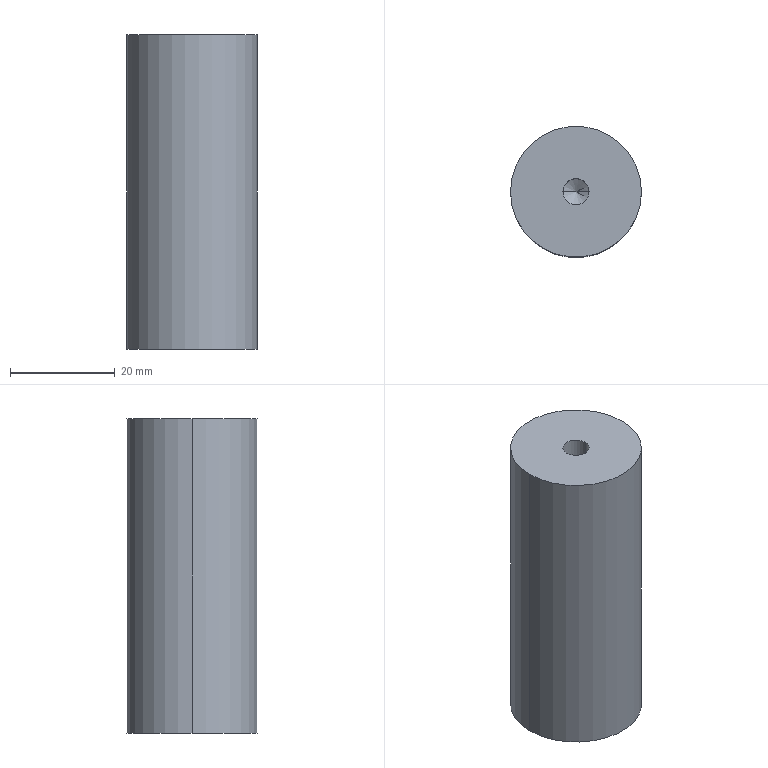Part | SolidWorks | features HoleWzd 2, Extrusion 1 | 1 solid | 12 faces | box 25 x 25 x 60 mm | volume 28844 mm3 | cylinder 6 | cone 4 | plane 2 | commonest cylinder face diameters 5 x4 25 x2
STEP:
#1=CARTESIAN_POINT('',(2.5,0.,15.));
#2=VERTEX_POINT('',#1);
#3=CARTESIAN_POINT('',(-2.5,0.,15.));
#4=VERTEX_POINT('',#3);
#5=CARTESIAN_POINT('',(0.,0.,15.));
#6=DIRECTION('',(0.,0.,-1.));
#7=DIRECTION('',(-1.,0.,0.));
#8=AXIS2_PLACEMENT_3D('',#5,#6,#7);
#9=CIRCLE('',#8,2.5);
#10=EDGE_CURVE('',#2,#4,#9,.T.);
#11=ORIENTED_EDGE('',*,*,#10,.F.);
#12=CARTESIAN_POINT('',(2.5,0.,0.));
#13=VERTEX_POINT('',#12);
#14=CARTESIAN_POINT('',(2.5,0.,0.));
#15=DIRECTION('',(0.,0.,-1.));
#16=VECTOR('',#15,1000.);
#17=LINE('',#14,#16);
#18=EDGE_CURVE('',#2,#13,#17,.T.);
#19=ORIENTED_EDGE('',*,*,#18,.T.);
#20=CARTESIAN_POINT('',(-2.5,0.,0.));
#21=VERTEX_POINT('',#20);
#22=CARTESIAN_POINT('',(0.,0.,0.));
#23=DIRECTION('',(0.,0.,-1.));
#24=DIRECTION('',(-1.,0.,0.));
#25=AXIS2_PLACEMENT_3D('',#22,#23,#24);
#26=CIRCLE('',#25,2.5);
#27=EDGE_CURVE('',#13,#21,#26,.T.);
#28=ORIENTED_EDGE('',*,*,#27,.T.);
#29=CARTESIAN_POINT('',(-2.5,0.,0.));
#30=DIRECTION('',(0.,0.,-1.));
#31=VECTOR('',#30,1000.);
#32=LINE('',#29,#31);
#33=EDGE_CURVE('',#4,#21,#32,.T.);
#34=ORIENTED_EDGE('',*,*,#33,.F.);
#35=EDGE_LOOP('',(#11,#19,#28,#34));
#36=FACE_OUTER_BOUND('',#35,.T.);
#37=CARTESIAN_POINT('',(0.,0.,0.));
#38=DIRECTION('',(0.,0.,-1.));
#39=DIRECTION('',(-1.,0.,0.));
#40=AXIS2_PLACEMENT_3D('',#37,#38,#39);
#41=CYLINDRICAL_SURFACE('',#40,2.5);
#42=ADVANCED_FACE('',(#36),#41,.F.);
#43=CARTESIAN_POINT('',(0.,0.,16.502));
#44=VERTEX_POINT('',#43);
#45=CARTESIAN_POINT('',(-2.5,0.,15.));
#46=DIRECTION('',(-0.8572,0.,-0.515));
#47=VECTOR('',#46,1000.);
#48=LINE('',#45,#47);
#49=EDGE_CURVE('',#44,#4,#48,.T.);
#50=ORIENTED_EDGE('',*,*,#49,.F.);
#51=CARTESIAN_POINT('',(2.5,0.,15.));
#52=DIRECTION('',(0.8572,0.,-0.515));
#53=VECTOR('',#52,1000.);
#54=LINE('',#51,#53);
#55=EDGE_CURVE('',#44,#2,#54,.T.);
#56=ORIENTED_EDGE('',*,*,#55,.T.);
#57=ORIENTED_EDGE('',*,*,#10,.T.);
#58=EDGE_LOOP('',(#50,#56,#57));
#59=FACE_OUTER_BOUND('',#58,.T.);
#60=CARTESIAN_POINT('',(0.,0.,15.));
#61=DIRECTION('',(0.,0.,-1.));
#62=DIRECTION('',(-1.,0.,0.));
#63=AXIS2_PLACEMENT_3D('',#60,#61,#62);
#64=CONICAL_SURFACE('',#63,2.5,1.03);
#65=ADVANCED_FACE('',(#59),#64,.F.);
#66=CARTESIAN_POINT('',(-2.5,0.,45.));
#67=VERTEX_POINT('',#66);
#68=CARTESIAN_POINT('',(2.5,0.,45.));
#69=VERTEX_POINT('',#68);
#70=CARTESIAN_POINT('',(0.,0.,45.));
#71=DIRECTION('',(0.,0.,1.));
#72=DIRECTION('',(1.,0.,0.));
#73=AXIS2_PLACEMENT_3D('',#70,#71,#72);
#74=CIRCLE('',#73,2.5);
#75=EDGE_CURVE('',#67,#69,#74,.T.);
#76=ORIENTED_EDGE('',*,*,#75,.F.);
#77=CARTESIAN_POINT('',(-2.5,0.,60.));
#78=VERTEX_POINT('',#77);
#79=CARTESIAN_POINT('',(-2.5,0.,60.));
#80=DIRECTION('',(0.,0.,1.));
#81=VECTOR('',#80,1000.);
#82=LINE('',#79,#81);
#83=EDGE_CURVE('',#67,#78,#82,.T.);
#84=ORIENTED_EDGE('',*,*,#83,.T.);
#85=CARTESIAN_POINT('',(2.5,0.,60.));
#86=VERTEX_POINT('',#85);
#87=CARTESIAN_POINT('',(0.,0.,60.));
#88=DIRECTION('',(0.,0.,1.));
#89=DIRECTION('',(1.,0.,0.));
#90=AXIS2_PLACEMENT_3D('',#87,#88,#89);
#91=CIRCLE('',#90,2.5);
#92=EDGE_CURVE('',#78,#86,#91,.T.);
#93=ORIENTED_EDGE('',*,*,#92,.T.);
#94=CARTESIAN_POINT('',(2.5,0.,60.));
#95=DIRECTION('',(0.,0.,1.));
#96=VECTOR('',#95,1000.);
#97=LINE('',#94,#96);
#98=EDGE_CURVE('',#69,#86,#97,.T.);
#99=ORIENTED_EDGE('',*,*,#98,.F.);
#100=EDGE_LOOP('',(#76,#84,#93,#99));
#101=FACE_OUTER_BOUND('',#100,.T.);
#102=CARTESIAN_POINT('',(0.,0.,60.));
#103=DIRECTION('',(0.,0.,1.));
#104=DIRECTION('',(1.,0.,0.));
#105=AXIS2_PLACEMENT_3D('',#102,#103,#104);
#106=CYLINDRICAL_SURFACE('',#105,2.5);
#107=ADVANCED_FACE('',(#101),#106,.F.);
#108=CARTESIAN_POINT('',(0.,0.,43.498));
#109=VERTEX_POINT('',#108);
#110=CARTESIAN_POINT('',(2.5,0.,45.));
#111=DIRECTION('',(0.8572,0.,0.515));
#112=VECTOR('',#111,1000.);
#113=LINE('',#110,#112);
#114=EDGE_CURVE('',#109,#69,#113,.T.);
#115=ORIENTED_EDGE('',*,*,#114,.F.);
#116=CARTESIAN_POINT('',(-2.5,0.,45.));
#117=DIRECTION('',(-0.8572,0.,0.515));
#118=VECTOR('',#117,1000.);
#119=LINE('',#116,#118);
#120=EDGE_CURVE('',#109,#67,#119,.T.);
#121=ORIENTED_EDGE('',*,*,#120,.T.);
#122=ORIENTED_EDGE('',*,*,#75,.T.);
#123=EDGE_LOOP('',(#115,#121,#122));
#124=FACE_OUTER_BOUND('',#123,.T.);
#125=CARTESIAN_POINT('',(0.,0.,45.));
#126=DIRECTION('',(0.,0.,1.));
#127=DIRECTION('',(1.,0.,0.));
#128=AXIS2_PLACEMENT_3D('',#125,#126,#127);
#129=CONICAL_SURFACE('',#128,2.5,1.03);
#130=ADVANCED_FACE('',(#124),#129,.F.);
#131=CARTESIAN_POINT('',(12.5,0.,60.));
#132=VERTEX_POINT('',#131);
#133=CARTESIAN_POINT('',(-12.5,0.,60.));
#134=VERTEX_POINT('',#133);
#135=CARTESIAN_POINT('',(0.,0.,60.));
#136=DIRECTION('',(0.,0.,1.));
#137=DIRECTION('',(1.,0.,0.));
#138=AXIS2_PLACEMENT_3D('',#135,#136,#137);
#139=CIRCLE('',#138,12.5);
#140=EDGE_CURVE('',#132,#134,#139,.T.);
#141=ORIENTED_EDGE('',*,*,#140,.F.);
#142=CARTESIAN_POINT('',(12.5,0.,0.));
#143=VERTEX_POINT('',#142);
#144=CARTESIAN_POINT('',(12.5,0.,60.));
#145=DIRECTION('',(0.,0.,-1.));
#146=VECTOR('',#145,1000.);
#147=LINE('',#144,#146);
#148=EDGE_CURVE('',#132,#143,#147,.T.);
#149=ORIENTED_EDGE('',*,*,#148,.T.);
#150=CARTESIAN_POINT('',(-12.5,0.,0.));
#151=VERTEX_POINT('',#150);
#152=CARTESIAN_POINT('',(0.,0.,0.));
#153=DIRECTION('',(0.,0.,1.));
#154=DIRECTION('',(1.,0.,0.));
#155=AXIS2_PLACEMENT_3D('',#152,#153,#154);
#156=CIRCLE('',#155,12.5);
#157=EDGE_CURVE('',#143,#151,#156,.T.);
#158=ORIENTED_EDGE('',*,*,#157,.T.);
#159=CARTESIAN_POINT('',(-12.5,0.,60.));
#160=DIRECTION('',(0.,0.,-1.));
#161=VECTOR('',#160,1000.);
#162=LINE('',#159,#161);
#163=EDGE_CURVE('',#134,#151,#162,.T.);
#164=ORIENTED_EDGE('',*,*,#163,.F.);
#165=EDGE_LOOP('',(#141,#149,#158,#164));
#166=FACE_OUTER_BOUND('',#165,.T.);
#167=CARTESIAN_POINT('',(0.,0.,60.));
#168=DIRECTION('',(0.,0.,-1.));
#169=DIRECTION('',(-1.,0.,0.));
#170=AXIS2_PLACEMENT_3D('',#167,#168,#169);
#171=CYLINDRICAL_SURFACE('',#170,12.5);
#172=ADVANCED_FACE('',(#166),#171,.T.);
#173=ORIENTED_EDGE('',*,*,#148,.F.);
#174=CARTESIAN_POINT('',(0.,0.,60.));
#175=DIRECTION('',(0.,0.,1.));
#176=DIRECTION('',(1.,0.,0.));
#177=AXIS2_PLACEMENT_3D('',#174,#175,#176);
#178=CIRCLE('',#177,12.5);
#179=EDGE_CURVE('',#134,#132,#178,.T.);
#180=ORIENTED_EDGE('',*,*,#179,.F.);
#181=ORIENTED_EDGE('',*,*,#163,.T.);
#182=CARTESIAN_POINT('',(0.,0.,0.));
#183=DIRECTION('',(0.,0.,1.));
#184=DIRECTION('',(1.,0.,0.));
#185=AXIS2_PLACEMENT_3D('',#182,#183,#184);
#186=CIRCLE('',#185,12.5);
#187=EDGE_CURVE('',#151,#143,#186,.T.);
#188=ORIENTED_EDGE('',*,*,#187,.T.);
#189=EDGE_LOOP('',(#173,#180,#181,#188));
#190=FACE_OUTER_BOUND('',#189,.T.);
#191=CARTESIAN_POINT('',(0.,0.,60.));
#192=DIRECTION('',(0.,0.,-1.));
#193=DIRECTION('',(-1.,0.,0.));
#194=AXIS2_PLACEMENT_3D('',#191,#192,#193);
#195=CYLINDRICAL_SURFACE('',#194,12.5);
#196=ADVANCED_FACE('',(#190),#195,.T.);
#197=CARTESIAN_POINT('',(0.,0.,60.));
#198=DIRECTION('',(0.,0.,1.));
#199=DIRECTION('',(1.,0.,0.));
#200=AXIS2_PLACEMENT_3D('',#197,#198,#199);
#201=CIRCLE('',#200,2.5);
#202=EDGE_CURVE('',#86,#78,#201,.T.);
#203=ORIENTED_EDGE('',*,*,#202,.F.);
#204=ORIENTED_EDGE('',*,*,#92,.F.);
#205=EDGE_LOOP('',(#203,#204));
#206=FACE_BOUND('',#205,.T.);
#207=ORIENTED_EDGE('',*,*,#179,.T.);
#208=ORIENTED_EDGE('',*,*,#140,.T.);
#209=EDGE_LOOP('',(#207,#208));
#210=FACE_OUTER_BOUND('',#209,.T.);
#211=CARTESIAN_POINT('',(0.,0.,60.));
#212=DIRECTION('',(0.,0.,1.));
#213=DIRECTION('',(1.,0.,0.));
#214=AXIS2_PLACEMENT_3D('',#211,#212,#213);
#215=PLANE('',#214);
#216=ADVANCED_FACE('',(#206,#210),#215,.T.);
#217=CARTESIAN_POINT('',(0.,0.,0.));
#218=DIRECTION('',(0.,0.,-1.));
#219=DIRECTION('',(-1.,0.,0.));
#220=AXIS2_PLACEMENT_3D('',#217,#218,#219);
#221=CIRCLE('',#220,2.5);
#222=EDGE_CURVE('',#21,#13,#221,.T.);
#223=ORIENTED_EDGE('',*,*,#222,.F.);
#224=ORIENTED_EDGE('',*,*,#27,.F.);
#225=EDGE_LOOP('',(#223,#224));
#226=FACE_BOUND('',#225,.T.);
#227=ORIENTED_EDGE('',*,*,#187,.F.);
#228=ORIENTED_EDGE('',*,*,#157,.F.);
#229=EDGE_LOOP('',(#227,#228));
#230=FACE_OUTER_BOUND('',#229,.T.);
#231=CARTESIAN_POINT('',(0.,0.,0.));
#232=DIRECTION('',(0.,0.,1.));
#233=DIRECTION('',(1.,0.,0.));
#234=AXIS2_PLACEMENT_3D('',#231,#232,#233);
#235=PLANE('',#234);
#236=ADVANCED_FACE('',(#226,#230),#235,.F.);
#237=ORIENTED_EDGE('',*,*,#120,.F.);
#238=ORIENTED_EDGE('',*,*,#114,.T.);
#239=CARTESIAN_POINT('',(0.,0.,45.));
#240=DIRECTION('',(0.,0.,1.));
#241=DIRECTION('',(1.,0.,0.));
#242=AXIS2_PLACEMENT_3D('',#239,#240,#241);
#243=CIRCLE('',#242,2.5);
#244=EDGE_CURVE('',#69,#67,#243,.T.);
#245=ORIENTED_EDGE('',*,*,#244,.T.);
#246=EDGE_LOOP('',(#237,#238,#245));
#247=FACE_OUTER_BOUND('',#246,.T.);
#248=CARTESIAN_POINT('',(0.,0.,45.));
#249=DIRECTION('',(0.,0.,1.));
#250=DIRECTION('',(1.,0.,0.));
#251=AXIS2_PLACEMENT_3D('',#248,#249,#250);
#252=CONICAL_SURFACE('',#251,2.5,1.03);
#253=ADVANCED_FACE('',(#247),#252,.F.);
#254=ORIENTED_EDGE('',*,*,#83,.F.);
#255=ORIENTED_EDGE('',*,*,#244,.F.);
#256=ORIENTED_EDGE('',*,*,#98,.T.);
#257=ORIENTED_EDGE('',*,*,#202,.T.);
#258=EDGE_LOOP('',(#254,#255,#256,#257));
#259=FACE_OUTER_BOUND('',#258,.T.);
#260=CARTESIAN_POINT('',(0.,0.,60.));
#261=DIRECTION('',(0.,0.,1.));
#262=DIRECTION('',(1.,0.,0.));
#263=AXIS2_PLACEMENT_3D('',#260,#261,#262);
#264=CYLINDRICAL_SURFACE('',#263,2.5);
#265=ADVANCED_FACE('',(#259),#264,.F.);
#266=ORIENTED_EDGE('',*,*,#55,.F.);
#267=ORIENTED_EDGE('',*,*,#49,.T.);
#268=CARTESIAN_POINT('',(0.,0.,15.));
#269=DIRECTION('',(0.,0.,-1.));
#270=DIRECTION('',(-1.,0.,0.));
#271=AXIS2_PLACEMENT_3D('',#268,#269,#270);
#272=CIRCLE('',#271,2.5);
#273=EDGE_CURVE('',#4,#2,#272,.T.);
#274=ORIENTED_EDGE('',*,*,#273,.T.);
#275=EDGE_LOOP('',(#266,#267,#274));
#276=FACE_OUTER_BOUND('',#275,.T.);
#277=CARTESIAN_POINT('',(0.,0.,15.));
#278=DIRECTION('',(0.,0.,-1.));
#279=DIRECTION('',(-1.,0.,0.));
#280=AXIS2_PLACEMENT_3D('',#277,#278,#279);
#281=CONICAL_SURFACE('',#280,2.5,1.03);
#282=ADVANCED_FACE('',(#276),#281,.F.);
#283=ORIENTED_EDGE('',*,*,#18,.F.);
#284=ORIENTED_EDGE('',*,*,#273,.F.);
#285=ORIENTED_EDGE('',*,*,#33,.T.);
#286=ORIENTED_EDGE('',*,*,#222,.T.);
#287=EDGE_LOOP('',(#283,#284,#285,#286));
#288=FACE_OUTER_BOUND('',#287,.T.);
#289=CARTESIAN_POINT('',(0.,0.,0.));
#290=DIRECTION('',(0.,0.,-1.));
#291=DIRECTION('',(-1.,0.,0.));
#292=AXIS2_PLACEMENT_3D('',#289,#290,#291);
#293=CYLINDRICAL_SURFACE('',#292,2.5);
#294=ADVANCED_FACE('',(#288),#293,.F.);
#295=CLOSED_SHELL('',(#42,#65,#107,#130,#172,#196,#216,#236,#253,#265,#282,#294));
#296=MANIFOLD_SOLID_BREP('',#295);
#297=CARTESIAN_POINT('',(0.,0.,0.));
#298=DIRECTION('',(0.,0.,1.));
#299=DIRECTION('',(1.,0.,0.));
#300=AXIS2_PLACEMENT_3D('',#297,#298,#299);
#301=(LENGTH_UNIT()NAMED_UNIT(*)SI_UNIT(.MILLI.,.METRE.));
#302=UNCERTAINTY_MEASURE_WITH_UNIT(LENGTH_MEASURE(0.00001),#301,'','');
#303=(NAMED_UNIT(*)PLANE_ANGLE_UNIT()SI_UNIT($,.RADIAN.));
#304=(NAMED_UNIT(*)SI_UNIT($,.STERADIAN.)SOLID_ANGLE_UNIT());
#305=(GEOMETRIC_REPRESENTATION_CONTEXT(3)GLOBAL_UNCERTAINTY_ASSIGNED_CONTEXT((#302))GLOBAL_UNIT_ASSIGNED_CONTEXT((#301,#303,#304))REPRESENTATION_CONTEXT('',''));
#306=ADVANCED_BREP_SHAPE_REPRESENTATION('',(#296,#300),#305);